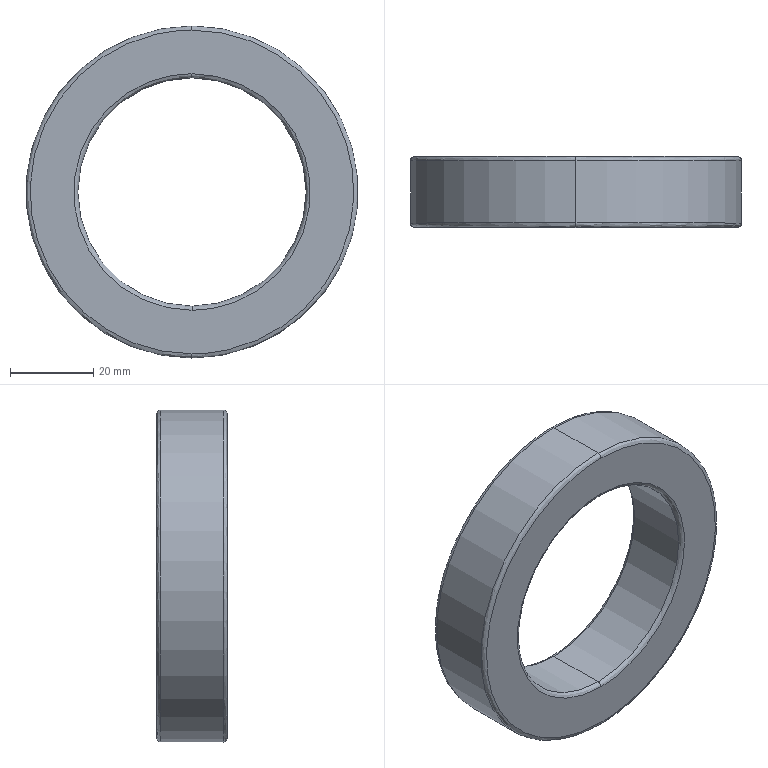Part | STEP file | Bearing 32911 | 1 solid | 14 faces | box 80 x 17 x 80 mm | volume 44892 mm3 | spline 8 | cylinder 4 | plane 2 | commonest cylinder face diameters 55 x2 80 x2